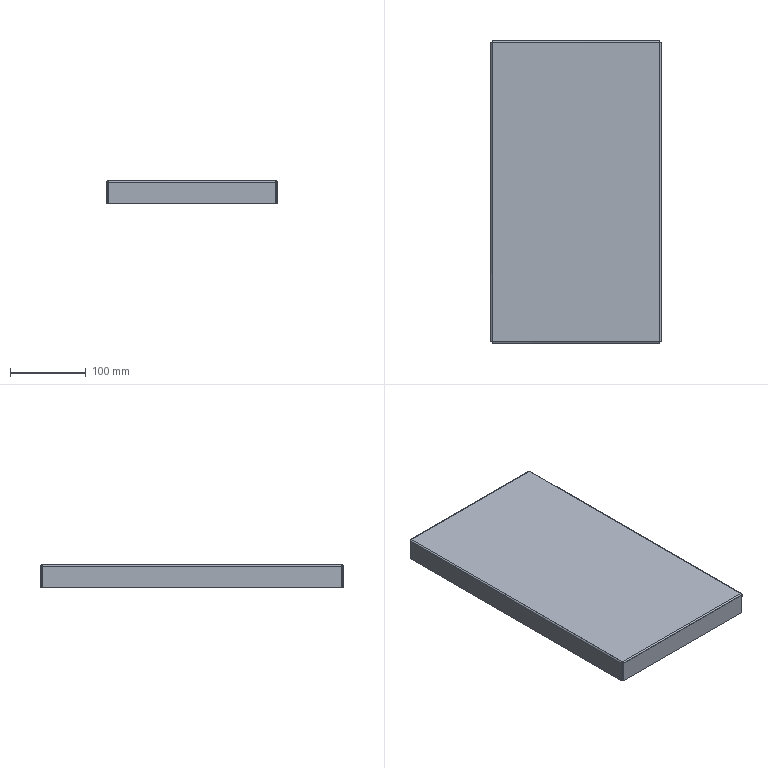Part | 1 solid | 38 faces | box 225 x 400 x 30 mm | volume 149808 mm3 | plane 22 | spline 8 | cylinder 8 | commonest cylinder face diameters 1.465 x4 3.865 x4
STEP:
#1=CARTESIAN_POINT('',(-110.567,-198.067,-1.2));
#2=VERTEX_POINT('',#1);
#3=CARTESIAN_POINT('',(110.567,-198.067,-1.2));
#4=VERTEX_POINT('',#3);
#5=CARTESIAN_POINT('',(-110.593,-198.067,-1.2));
#6=DIRECTION('',(1.,0.,0.));
#7=VECTOR('',#6,1000.);
#8=LINE('',#5,#7);
#9=EDGE_CURVE('',#2,#4,#8,.T.);
#10=ORIENTED_EDGE('',*,*,#9,.F.);
#11=CARTESIAN_POINT('',(-110.567,198.067,-1.2));
#12=VERTEX_POINT('',#11);
#13=CARTESIAN_POINT('',(-110.567,198.093,-1.2));
#14=DIRECTION('',(0.,-1.,0.));
#15=VECTOR('',#14,1000.);
#16=LINE('',#13,#15);
#17=EDGE_CURVE('',#12,#2,#16,.T.);
#18=ORIENTED_EDGE('',*,*,#17,.F.);
#19=CARTESIAN_POINT('',(110.567,198.067,-1.2));
#20=VERTEX_POINT('',#19);
#21=CARTESIAN_POINT('',(110.593,198.067,-1.2));
#22=DIRECTION('',(-1.,0.,0.));
#23=VECTOR('',#22,1000.);
#24=LINE('',#21,#23);
#25=EDGE_CURVE('',#20,#12,#24,.T.);
#26=ORIENTED_EDGE('',*,*,#25,.F.);
#27=CARTESIAN_POINT('',(110.567,-198.093,-1.2));
#28=DIRECTION('',(0.,1.,0.));
#29=VECTOR('',#28,1000.);
#30=LINE('',#27,#29);
#31=EDGE_CURVE('',#4,#20,#30,.T.);
#32=ORIENTED_EDGE('',*,*,#31,.F.);
#33=EDGE_LOOP('',(#10,#18,#26,#32));
#34=FACE_OUTER_BOUND('',#33,.T.);
#35=CARTESIAN_POINT('',(0.,0.,-1.2));
#36=DIRECTION('',(0.,0.,1.));
#37=DIRECTION('',(1.,0.,0.));
#38=AXIS2_PLACEMENT_3D('',#35,#36,#37);
#39=PLANE('',#38);
#40=ADVANCED_FACE('',(#34),#39,.F.);
#41=CARTESIAN_POINT('',(-110.567,198.067,0.));
#42=VERTEX_POINT('',#41);
#43=CARTESIAN_POINT('',(-110.567,-198.067,0.));
#44=VERTEX_POINT('',#43);
#45=CARTESIAN_POINT('',(-110.567,198.093,0.));
#46=DIRECTION('',(0.,-1.,0.));
#47=VECTOR('',#46,1000.);
#48=LINE('',#45,#47);
#49=EDGE_CURVE('',#42,#44,#48,.T.);
#50=ORIENTED_EDGE('',*,*,#49,.T.);
#51=CARTESIAN_POINT('',(110.567,-198.067,0.));
#52=VERTEX_POINT('',#51);
#53=CARTESIAN_POINT('',(-110.593,-198.067,0.));
#54=DIRECTION('',(1.,0.,0.));
#55=VECTOR('',#54,1000.);
#56=LINE('',#53,#55);
#57=EDGE_CURVE('',#44,#52,#56,.T.);
#58=ORIENTED_EDGE('',*,*,#57,.T.);
#59=CARTESIAN_POINT('',(110.567,198.067,0.));
#60=VERTEX_POINT('',#59);
#61=CARTESIAN_POINT('',(110.567,-198.093,0.));
#62=DIRECTION('',(0.,1.,0.));
#63=VECTOR('',#62,1000.);
#64=LINE('',#61,#63);
#65=EDGE_CURVE('',#52,#60,#64,.T.);
#66=ORIENTED_EDGE('',*,*,#65,.T.);
#67=CARTESIAN_POINT('',(110.593,198.067,0.));
#68=DIRECTION('',(-1.,0.,0.));
#69=VECTOR('',#68,1000.);
#70=LINE('',#67,#69);
#71=EDGE_CURVE('',#60,#42,#70,.T.);
#72=ORIENTED_EDGE('',*,*,#71,.T.);
#73=EDGE_LOOP('',(#50,#58,#66,#72));
#74=FACE_OUTER_BOUND('',#73,.T.);
#75=CARTESIAN_POINT('',(0.,0.,0.));
#76=DIRECTION('',(0.,0.,1.));
#77=DIRECTION('',(1.,0.,0.));
#78=AXIS2_PLACEMENT_3D('',#75,#76,#77);
#79=PLANE('',#78);
#80=ADVANCED_FACE('',(#74),#79,.T.);
#81=CARTESIAN_POINT('',(112.5,198.093,-1.933));
#82=VERTEX_POINT('',#81);
#83=CARTESIAN_POINT('',(111.3,198.093,-1.933));
#84=VERTEX_POINT('',#83);
#85=CARTESIAN_POINT('',(111.3,198.093,-1.933));
#86=DIRECTION('',(-1.,0.,0.));
#87=VECTOR('',#86,1000.);
#88=LINE('',#85,#87);
#89=EDGE_CURVE('',#82,#84,#88,.T.);
#90=ORIENTED_EDGE('',*,*,#89,.T.);
#91=CARTESIAN_POINT('',(110.567,198.067,-1.2));
#92=CARTESIAN_POINT('',(110.759,198.072,-1.2));
#93=CARTESIAN_POINT('',(110.95,198.076,-1.279));
#94=CARTESIAN_POINT('',(111.221,198.084,-1.55));
#95=CARTESIAN_POINT('',(111.3,198.089,-1.741));
#96=CARTESIAN_POINT('',(111.3,198.093,-1.933));
#97=B_SPLINE_CURVE_WITH_KNOTS('',3,(#91,#92,#93,#94,#95,#96),.UNSPECIFIED.,.F.,.F.,(4,2,4),(0.,0.5,1.),.UNSPECIFIED.);
#98=EDGE_CURVE('',#20,#84,#97,.T.);
#99=ORIENTED_EDGE('',*,*,#98,.F.);
#100=CARTESIAN_POINT('',(110.567,198.067,-1.2));
#101=DIRECTION('',(0.,0.,1.));
#102=VECTOR('',#101,1000.);
#103=LINE('',#100,#102);
#104=EDGE_CURVE('',#20,#60,#103,.T.);
#105=ORIENTED_EDGE('',*,*,#104,.T.);
#106=CARTESIAN_POINT('',(110.567,198.067,0.));
#107=CARTESIAN_POINT('',(110.82,198.07,0.));
#108=CARTESIAN_POINT('',(111.073,198.072,-0.0503));
#109=CARTESIAN_POINT('',(111.541,198.076,-0.2439));
#110=CARTESIAN_POINT('',(111.755,198.078,-0.3872));
#111=CARTESIAN_POINT('',(112.113,198.082,-0.7449));
#112=CARTESIAN_POINT('',(112.256,198.084,-0.9593));
#113=CARTESIAN_POINT('',(112.45,198.089,-1.427));
#114=CARTESIAN_POINT('',(112.5,198.091,-1.68));
#115=CARTESIAN_POINT('',(112.5,198.093,-1.933));
#116=B_SPLINE_CURVE_WITH_KNOTS('',3,(#106,#107,#108,#109,#110,#111,#112,#113,#114,#115),.UNSPECIFIED.,.F.,.F.,(4,2,2,2,4),(0.,0.25,0.5,0.75,1.),.UNSPECIFIED.);
#117=EDGE_CURVE('',#60,#82,#116,.T.);
#118=ORIENTED_EDGE('',*,*,#117,.T.);
#119=EDGE_LOOP('',(#90,#99,#105,#118));
#120=FACE_OUTER_BOUND('',#119,.T.);
#121=CARTESIAN_POINT('',(110.567,198.067,0.012));
#122=CARTESIAN_POINT('',(110.822,198.07,0.012));
#123=CARTESIAN_POINT('',(111.076,198.072,-0.03861));
#124=CARTESIAN_POINT('',(111.547,198.076,-0.2334));
#125=CARTESIAN_POINT('',(111.762,198.078,-0.3776));
#126=CARTESIAN_POINT('',(112.122,198.082,-0.7376));
#127=CARTESIAN_POINT('',(112.267,198.084,-0.9533));
#128=CARTESIAN_POINT('',(112.461,198.089,-1.424));
#129=CARTESIAN_POINT('',(112.512,198.091,-1.678));
#130=CARTESIAN_POINT('',(112.512,198.093,-1.933));
#131=CARTESIAN_POINT('',(110.567,198.067,0.));
#132=CARTESIAN_POINT('',(110.82,198.07,0.));
#133=CARTESIAN_POINT('',(111.073,198.072,-0.0503));
#134=CARTESIAN_POINT('',(111.541,198.076,-0.2439));
#135=CARTESIAN_POINT('',(111.755,198.078,-0.3872));
#136=CARTESIAN_POINT('',(112.113,198.082,-0.7449));
#137=CARTESIAN_POINT('',(112.256,198.084,-0.9593));
#138=CARTESIAN_POINT('',(112.45,198.089,-1.427));
#139=CARTESIAN_POINT('',(112.5,198.091,-1.68));
#140=CARTESIAN_POINT('',(112.5,198.093,-1.933));
#141=CARTESIAN_POINT('',(110.567,198.067,-1.2));
#142=CARTESIAN_POINT('',(110.663,198.07,-1.2));
#143=CARTESIAN_POINT('',(110.759,198.072,-1.219));
#144=CARTESIAN_POINT('',(110.936,198.076,-1.292));
#145=CARTESIAN_POINT('',(111.018,198.078,-1.347));
#146=CARTESIAN_POINT('',(111.153,198.082,-1.482));
#147=CARTESIAN_POINT('',(111.208,198.084,-1.564));
#148=CARTESIAN_POINT('',(111.281,198.089,-1.741));
#149=CARTESIAN_POINT('',(111.3,198.091,-1.837));
#150=CARTESIAN_POINT('',(111.3,198.093,-1.933));
#151=CARTESIAN_POINT('',(110.567,198.067,-1.212));
#152=CARTESIAN_POINT('',(110.662,198.07,-1.212));
#153=CARTESIAN_POINT('',(110.756,198.072,-1.231));
#154=CARTESIAN_POINT('',(110.93,198.076,-1.303));
#155=CARTESIAN_POINT('',(111.01,198.078,-1.356));
#156=CARTESIAN_POINT('',(111.144,198.082,-1.49));
#157=CARTESIAN_POINT('',(111.197,198.084,-1.57));
#158=CARTESIAN_POINT('',(111.269,198.089,-1.744));
#159=CARTESIAN_POINT('',(111.288,198.091,-1.838));
#160=CARTESIAN_POINT('',(111.288,198.093,-1.933));
#161=B_SPLINE_SURFACE_WITH_KNOTS('',1,3,((#121,#122,#123,#124,#125,#126,#127,#128,#129,#130),(#131,#132,#133,#134,#135,#136,#137,#138,#139,#140),(#141,#142,#143,#144,#145,#146,#147,#148,#149,#150),(#151,#152,#153,#154,#155,#156,#157,#158,#159,#160)),.UNSPECIFIED.,.F.,.F.,.F.,(2,1,1,2),(4,2,2,2,4),(-0.01,0.,1.,1.01),(0.,0.25,0.5,0.75,1.),.UNSPECIFIED.);
#162=ADVANCED_FACE('',(#120),#161,.F.);
#163=CARTESIAN_POINT('',(111.3,-198.093,-1.933));
#164=VERTEX_POINT('',#163);
#165=CARTESIAN_POINT('',(111.3,-198.093,-1.933));
#166=CARTESIAN_POINT('',(111.3,-198.089,-1.741));
#167=CARTESIAN_POINT('',(111.221,-198.084,-1.55));
#168=CARTESIAN_POINT('',(110.95,-198.076,-1.279));
#169=CARTESIAN_POINT('',(110.759,-198.072,-1.2));
#170=CARTESIAN_POINT('',(110.567,-198.067,-1.2));
#171=B_SPLINE_CURVE_WITH_KNOTS('',3,(#165,#166,#167,#168,#169,#170),.UNSPECIFIED.,.F.,.F.,(4,2,4),(0.,0.5,1.),.UNSPECIFIED.);
#172=EDGE_CURVE('',#164,#4,#171,.T.);
#173=ORIENTED_EDGE('',*,*,#172,.F.);
#174=CARTESIAN_POINT('',(112.5,-198.093,-1.933));
#175=VERTEX_POINT('',#174);
#176=CARTESIAN_POINT('',(111.3,-198.093,-1.933));
#177=DIRECTION('',(-1.,0.,0.));
#178=VECTOR('',#177,1000.);
#179=LINE('',#176,#178);
#180=EDGE_CURVE('',#175,#164,#179,.T.);
#181=ORIENTED_EDGE('',*,*,#180,.F.);
#182=CARTESIAN_POINT('',(112.5,-198.093,-1.933));
#183=CARTESIAN_POINT('',(112.5,-198.091,-1.68));
#184=CARTESIAN_POINT('',(112.45,-198.089,-1.427));
#185=CARTESIAN_POINT('',(112.256,-198.084,-0.9593));
#186=CARTESIAN_POINT('',(112.113,-198.082,-0.7449));
#187=CARTESIAN_POINT('',(111.755,-198.078,-0.3872));
#188=CARTESIAN_POINT('',(111.541,-198.076,-0.2439));
#189=CARTESIAN_POINT('',(111.073,-198.072,-0.0503));
#190=CARTESIAN_POINT('',(110.82,-198.07,0.));
#191=CARTESIAN_POINT('',(110.567,-198.067,0.));
#192=B_SPLINE_CURVE_WITH_KNOTS('',3,(#182,#183,#184,#185,#186,#187,#188,#189,#190,#191),.UNSPECIFIED.,.F.,.F.,(4,2,2,2,4),(0.,0.25,0.5,0.75,1.),.UNSPECIFIED.);
#193=EDGE_CURVE('',#175,#52,#192,.T.);
#194=ORIENTED_EDGE('',*,*,#193,.T.);
#195=CARTESIAN_POINT('',(110.567,-198.067,-1.2));
#196=DIRECTION('',(0.,0.,1.));
#197=VECTOR('',#196,1000.);
#198=LINE('',#195,#197);
#199=EDGE_CURVE('',#4,#52,#198,.T.);
#200=ORIENTED_EDGE('',*,*,#199,.F.);
#201=EDGE_LOOP('',(#173,#181,#194,#200));
#202=FACE_OUTER_BOUND('',#201,.T.);
#203=CARTESIAN_POINT('',(112.512,-198.093,-1.933));
#204=CARTESIAN_POINT('',(112.512,-198.091,-1.678));
#205=CARTESIAN_POINT('',(112.461,-198.089,-1.424));
#206=CARTESIAN_POINT('',(112.267,-198.084,-0.9533));
#207=CARTESIAN_POINT('',(112.122,-198.082,-0.7376));
#208=CARTESIAN_POINT('',(111.762,-198.078,-0.3776));
#209=CARTESIAN_POINT('',(111.547,-198.076,-0.2334));
#210=CARTESIAN_POINT('',(111.076,-198.072,-0.03861));
#211=CARTESIAN_POINT('',(110.822,-198.07,0.012));
#212=CARTESIAN_POINT('',(110.567,-198.067,0.012));
#213=CARTESIAN_POINT('',(112.5,-198.093,-1.933));
#214=CARTESIAN_POINT('',(112.5,-198.091,-1.68));
#215=CARTESIAN_POINT('',(112.45,-198.089,-1.427));
#216=CARTESIAN_POINT('',(112.256,-198.084,-0.9593));
#217=CARTESIAN_POINT('',(112.113,-198.082,-0.7449));
#218=CARTESIAN_POINT('',(111.755,-198.078,-0.3872));
#219=CARTESIAN_POINT('',(111.541,-198.076,-0.2439));
#220=CARTESIAN_POINT('',(111.073,-198.072,-0.0503));
#221=CARTESIAN_POINT('',(110.82,-198.07,0.));
#222=CARTESIAN_POINT('',(110.567,-198.067,0.));
#223=CARTESIAN_POINT('',(111.3,-198.093,-1.933));
#224=CARTESIAN_POINT('',(111.3,-198.091,-1.837));
#225=CARTESIAN_POINT('',(111.281,-198.089,-1.741));
#226=CARTESIAN_POINT('',(111.208,-198.084,-1.564));
#227=CARTESIAN_POINT('',(111.153,-198.082,-1.482));
#228=CARTESIAN_POINT('',(111.018,-198.078,-1.347));
#229=CARTESIAN_POINT('',(110.936,-198.076,-1.292));
#230=CARTESIAN_POINT('',(110.759,-198.072,-1.219));
#231=CARTESIAN_POINT('',(110.663,-198.07,-1.2));
#232=CARTESIAN_POINT('',(110.567,-198.067,-1.2));
#233=CARTESIAN_POINT('',(111.288,-198.093,-1.933));
#234=CARTESIAN_POINT('',(111.288,-198.091,-1.838));
#235=CARTESIAN_POINT('',(111.269,-198.089,-1.744));
#236=CARTESIAN_POINT('',(111.197,-198.084,-1.57));
#237=CARTESIAN_POINT('',(111.144,-198.082,-1.49));
#238=CARTESIAN_POINT('',(111.01,-198.078,-1.356));
#239=CARTESIAN_POINT('',(110.93,-198.076,-1.303));
#240=CARTESIAN_POINT('',(110.756,-198.072,-1.231));
#241=CARTESIAN_POINT('',(110.662,-198.07,-1.212));
#242=CARTESIAN_POINT('',(110.567,-198.067,-1.212));
#243=B_SPLINE_SURFACE_WITH_KNOTS('',1,3,((#203,#204,#205,#206,#207,#208,#209,#210,#211,#212),(#213,#214,#215,#216,#217,#218,#219,#220,#221,#222),(#223,#224,#225,#226,#227,#228,#229,#230,#231,#232),(#233,#234,#235,#236,#237,#238,#239,#240,#241,#242)),.UNSPECIFIED.,.F.,.F.,.F.,(2,1,1,2),(4,2,2,2,4),(-0.01,0.,1.,1.01),(0.,0.25,0.5,0.75,1.),.UNSPECIFIED.);
#244=ADVANCED_FACE('',(#202),#243,.F.);
#245=ORIENTED_EDGE('',*,*,#65,.F.);
#246=ORIENTED_EDGE('',*,*,#193,.F.);
#247=CARTESIAN_POINT('',(112.5,0.,-1.933));
#248=DIRECTION('',(0.,-1.,0.));
#249=VECTOR('',#248,1000.);
#250=LINE('',#247,#249);
#251=EDGE_CURVE('',#82,#175,#250,.T.);
#252=ORIENTED_EDGE('',*,*,#251,.F.);
#253=ORIENTED_EDGE('',*,*,#117,.F.);
#254=EDGE_LOOP('',(#245,#246,#252,#253));
#255=FACE_OUTER_BOUND('',#254,.T.);
#256=CARTESIAN_POINT('',(110.567,-198.093,-1.933));
#257=DIRECTION('',(0.,-1.,0.));
#258=DIRECTION('',(1.,0.,0.));
#259=AXIS2_PLACEMENT_3D('',#256,#257,#258);
#260=CYLINDRICAL_SURFACE('',#259,1.933);
#261=ADVANCED_FACE('',(#255),#260,.T.);
#262=ORIENTED_EDGE('',*,*,#31,.T.);
#263=ORIENTED_EDGE('',*,*,#98,.T.);
#264=CARTESIAN_POINT('',(111.3,200.,-1.933));
#265=DIRECTION('',(0.,-1.,0.));
#266=VECTOR('',#265,1000.);
#267=LINE('',#264,#266);
#268=EDGE_CURVE('',#84,#164,#267,.T.);
#269=ORIENTED_EDGE('',*,*,#268,.T.);
#270=ORIENTED_EDGE('',*,*,#172,.T.);
#271=EDGE_LOOP('',(#262,#263,#269,#270));
#272=FACE_OUTER_BOUND('',#271,.T.);
#273=CARTESIAN_POINT('',(110.567,-198.093,-1.933));
#274=DIRECTION('',(0.,-1.,0.));
#275=DIRECTION('',(1.,0.,0.));
#276=AXIS2_PLACEMENT_3D('',#273,#274,#275);
#277=CYLINDRICAL_SURFACE('',#276,0.7326);
#278=ADVANCED_FACE('',(#272),#277,.F.);
#279=CARTESIAN_POINT('',(111.3,198.093,-30.));
#280=VERTEX_POINT('',#279);
#281=CARTESIAN_POINT('',(112.5,198.093,-30.));
#282=VERTEX_POINT('',#281);
#283=CARTESIAN_POINT('',(112.5,198.093,-30.));
#284=DIRECTION('',(1.,0.,0.));
#285=VECTOR('',#284,1000.);
#286=LINE('',#283,#285);
#287=EDGE_CURVE('',#280,#282,#286,.T.);
#288=ORIENTED_EDGE('',*,*,#287,.F.);
#289=CARTESIAN_POINT('',(111.3,198.093,0.));
#290=DIRECTION('',(0.,0.,-1.));
#291=VECTOR('',#290,1000.);
#292=LINE('',#289,#291);
#293=EDGE_CURVE('',#84,#280,#292,.T.);
#294=ORIENTED_EDGE('',*,*,#293,.F.);
#295=ORIENTED_EDGE('',*,*,#89,.F.);
#296=CARTESIAN_POINT('',(112.5,198.093,0.));
#297=DIRECTION('',(0.,0.,1.));
#298=VECTOR('',#297,1000.);
#299=LINE('',#296,#298);
#300=EDGE_CURVE('',#282,#82,#299,.T.);
#301=ORIENTED_EDGE('',*,*,#300,.F.);
#302=EDGE_LOOP('',(#288,#294,#295,#301));
#303=FACE_OUTER_BOUND('',#302,.T.);
#304=CARTESIAN_POINT('',(111.3,198.093,-1.2));
#305=DIRECTION('',(0.,1.,0.));
#306=DIRECTION('',(0.,0.,-1.));
#307=AXIS2_PLACEMENT_3D('',#304,#305,#306);
#308=PLANE('',#307);
#309=ADVANCED_FACE('',(#303),#308,.T.);
#310=CARTESIAN_POINT('',(112.5,-198.093,-30.));
#311=VERTEX_POINT('',#310);
#312=CARTESIAN_POINT('',(112.5,-198.093,-1.2));
#313=DIRECTION('',(0.,0.,1.));
#314=VECTOR('',#313,1000.);
#315=LINE('',#312,#314);
#316=EDGE_CURVE('',#311,#175,#315,.T.);
#317=ORIENTED_EDGE('',*,*,#316,.F.);
#318=CARTESIAN_POINT('',(112.5,-200.,-30.));
#319=DIRECTION('',(0.,-1.,0.));
#320=VECTOR('',#319,1000.);
#321=LINE('',#318,#320);
#322=EDGE_CURVE('',#282,#311,#321,.T.);
#323=ORIENTED_EDGE('',*,*,#322,.F.);
#324=ORIENTED_EDGE('',*,*,#300,.T.);
#325=ORIENTED_EDGE('',*,*,#251,.T.);
#326=EDGE_LOOP('',(#317,#323,#324,#325));
#327=FACE_OUTER_BOUND('',#326,.T.);
#328=CARTESIAN_POINT('',(112.5,0.,0.));
#329=DIRECTION('',(1.,0.,0.));
#330=DIRECTION('',(0.,0.,1.));
#331=AXIS2_PLACEMENT_3D('',#328,#329,#330);
#332=PLANE('',#331);
#333=ADVANCED_FACE('',(#327),#332,.T.);
#334=CARTESIAN_POINT('',(111.3,-198.093,-30.));
#335=VERTEX_POINT('',#334);
#336=CARTESIAN_POINT('',(111.3,0.,-30.));
#337=DIRECTION('',(0.,-1.,0.));
#338=VECTOR('',#337,1000.);
#339=LINE('',#336,#338);
#340=EDGE_CURVE('',#280,#335,#339,.T.);
#341=ORIENTED_EDGE('',*,*,#340,.T.);
#342=CARTESIAN_POINT('',(111.3,-198.093,-1.2));
#343=DIRECTION('',(0.,0.,-1.));
#344=VECTOR('',#343,1000.);
#345=LINE('',#342,#344);
#346=EDGE_CURVE('',#164,#335,#345,.T.);
#347=ORIENTED_EDGE('',*,*,#346,.F.);
#348=ORIENTED_EDGE('',*,*,#268,.F.);
#349=ORIENTED_EDGE('',*,*,#293,.T.);
#350=EDGE_LOOP('',(#341,#347,#348,#349));
#351=FACE_OUTER_BOUND('',#350,.T.);
#352=CARTESIAN_POINT('',(111.3,0.,0.));
#353=DIRECTION('',(1.,0.,0.));
#354=DIRECTION('',(0.,0.,1.));
#355=AXIS2_PLACEMENT_3D('',#352,#353,#354);
#356=PLANE('',#355);
#357=ADVANCED_FACE('',(#351),#356,.F.);
#358=CARTESIAN_POINT('',(111.3,-198.093,-30.));
#359=DIRECTION('',(1.,0.,0.));
#360=VECTOR('',#359,1000.);
#361=LINE('',#358,#360);
#362=EDGE_CURVE('',#335,#311,#361,.T.);
#363=ORIENTED_EDGE('',*,*,#362,.F.);
#364=ORIENTED_EDGE('',*,*,#340,.F.);
#365=ORIENTED_EDGE('',*,*,#287,.T.);
#366=ORIENTED_EDGE('',*,*,#322,.T.);
#367=EDGE_LOOP('',(#363,#364,#365,#366));
#368=FACE_OUTER_BOUND('',#367,.T.);
#369=CARTESIAN_POINT('',(112.5,-200.,-30.));
#370=DIRECTION('',(0.,0.,-1.));
#371=DIRECTION('',(0.,-1.,0.));
#372=AXIS2_PLACEMENT_3D('',#369,#370,#371);
#373=PLANE('',#372);
#374=ADVANCED_FACE('',(#368),#373,.T.);
#375=ORIENTED_EDGE('',*,*,#346,.T.);
#376=ORIENTED_EDGE('',*,*,#362,.T.);
#377=ORIENTED_EDGE('',*,*,#316,.T.);
#378=ORIENTED_EDGE('',*,*,#180,.T.);
#379=EDGE_LOOP('',(#375,#376,#377,#378));
#380=FACE_OUTER_BOUND('',#379,.T.);
#381=CARTESIAN_POINT('',(111.3,-198.093,-1.2));
#382=DIRECTION('',(0.,1.,0.));
#383=DIRECTION('',(0.,0.,-1.));
#384=AXIS2_PLACEMENT_3D('',#381,#382,#383);
#385=PLANE('',#384);
#386=ADVANCED_FACE('',(#380),#385,.F.);
#387=CARTESIAN_POINT('',(-110.593,200.,-1.933));
#388=VERTEX_POINT('',#387);
#389=CARTESIAN_POINT('',(-110.593,198.8,-1.933));
#390=VERTEX_POINT('',#389);
#391=CARTESIAN_POINT('',(-110.593,198.8,-1.933));
#392=DIRECTION('',(0.,-1.,0.));
#393=VECTOR('',#392,1000.);
#394=LINE('',#391,#393);
#395=EDGE_CURVE('',#388,#390,#394,.T.);
#396=ORIENTED_EDGE('',*,*,#395,.T.);
#397=CARTESIAN_POINT('',(-110.567,198.067,-1.2));
#398=CARTESIAN_POINT('',(-110.572,198.259,-1.2));
#399=CARTESIAN_POINT('',(-110.576,198.45,-1.279));
#400=CARTESIAN_POINT('',(-110.584,198.721,-1.55));
#401=CARTESIAN_POINT('',(-110.589,198.8,-1.741));
#402=CARTESIAN_POINT('',(-110.593,198.8,-1.933));
#403=B_SPLINE_CURVE_WITH_KNOTS('',3,(#397,#398,#399,#400,#401,#402),.UNSPECIFIED.,.F.,.F.,(4,2,4),(0.,0.5,1.),.UNSPECIFIED.);
#404=EDGE_CURVE('',#12,#390,#403,.T.);
#405=ORIENTED_EDGE('',*,*,#404,.F.);
#406=CARTESIAN_POINT('',(-110.567,198.067,-1.2));
#407=DIRECTION('',(0.,0.,1.));
#408=VECTOR('',#407,1000.);
#409=LINE('',#406,#408);
#410=EDGE_CURVE('',#12,#42,#409,.T.);
#411=ORIENTED_EDGE('',*,*,#410,.T.);
#412=CARTESIAN_POINT('',(-110.567,198.067,0.));
#413=CARTESIAN_POINT('',(-110.57,198.32,0.));
#414=CARTESIAN_POINT('',(-110.572,198.573,-0.0503));
#415=CARTESIAN_POINT('',(-110.576,199.041,-0.2439));
#416=CARTESIAN_POINT('',(-110.578,199.255,-0.3872));
#417=CARTESIAN_POINT('',(-110.582,199.613,-0.7449));
#418=CARTESIAN_POINT('',(-110.584,199.756,-0.9593));
#419=CARTESIAN_POINT('',(-110.589,199.95,-1.427));
#420=CARTESIAN_POINT('',(-110.591,200.,-1.68));
#421=CARTESIAN_POINT('',(-110.593,200.,-1.933));
#422=B_SPLINE_CURVE_WITH_KNOTS('',3,(#412,#413,#414,#415,#416,#417,#418,#419,#420,#421),.UNSPECIFIED.,.F.,.F.,(4,2,2,2,4),(0.,0.25,0.5,0.75,1.),.UNSPECIFIED.);
#423=EDGE_CURVE('',#42,#388,#422,.T.);
#424=ORIENTED_EDGE('',*,*,#423,.T.);
#425=EDGE_LOOP('',(#396,#405,#411,#424));
#426=FACE_OUTER_BOUND('',#425,.T.);
#427=CARTESIAN_POINT('',(-110.567,198.067,0.012));
#428=CARTESIAN_POINT('',(-110.57,198.322,0.012));
#429=CARTESIAN_POINT('',(-110.572,198.576,-0.03861));
#430=CARTESIAN_POINT('',(-110.576,199.047,-0.2334));
#431=CARTESIAN_POINT('',(-110.578,199.262,-0.3776));
#432=CARTESIAN_POINT('',(-110.582,199.622,-0.7376));
#433=CARTESIAN_POINT('',(-110.584,199.767,-0.9533));
#434=CARTESIAN_POINT('',(-110.589,199.961,-1.424));
#435=CARTESIAN_POINT('',(-110.591,200.012,-1.678));
#436=CARTESIAN_POINT('',(-110.593,200.012,-1.933));
#437=CARTESIAN_POINT('',(-110.567,198.067,0.));
#438=CARTESIAN_POINT('',(-110.57,198.32,0.));
#439=CARTESIAN_POINT('',(-110.572,198.573,-0.0503));
#440=CARTESIAN_POINT('',(-110.576,199.041,-0.2439));
#441=CARTESIAN_POINT('',(-110.578,199.255,-0.3872));
#442=CARTESIAN_POINT('',(-110.582,199.613,-0.7449));
#443=CARTESIAN_POINT('',(-110.584,199.756,-0.9593));
#444=CARTESIAN_POINT('',(-110.589,199.95,-1.427));
#445=CARTESIAN_POINT('',(-110.591,200.,-1.68));
#446=CARTESIAN_POINT('',(-110.593,200.,-1.933));
#447=CARTESIAN_POINT('',(-110.567,198.067,-1.2));
#448=CARTESIAN_POINT('',(-110.57,198.163,-1.2));
#449=CARTESIAN_POINT('',(-110.572,198.259,-1.219));
#450=CARTESIAN_POINT('',(-110.576,198.436,-1.292));
#451=CARTESIAN_POINT('',(-110.578,198.518,-1.347));
#452=CARTESIAN_POINT('',(-110.582,198.653,-1.482));
#453=CARTESIAN_POINT('',(-110.584,198.708,-1.564));
#454=CARTESIAN_POINT('',(-110.589,198.781,-1.741));
#455=CARTESIAN_POINT('',(-110.591,198.8,-1.837));
#456=CARTESIAN_POINT('',(-110.593,198.8,-1.933));
#457=CARTESIAN_POINT('',(-110.567,198.067,-1.212));
#458=CARTESIAN_POINT('',(-110.57,198.162,-1.212));
#459=CARTESIAN_POINT('',(-110.572,198.256,-1.231));
#460=CARTESIAN_POINT('',(-110.576,198.43,-1.303));
#461=CARTESIAN_POINT('',(-110.578,198.51,-1.356));
#462=CARTESIAN_POINT('',(-110.582,198.644,-1.49));
#463=CARTESIAN_POINT('',(-110.584,198.697,-1.57));
#464=CARTESIAN_POINT('',(-110.589,198.769,-1.744));
#465=CARTESIAN_POINT('',(-110.591,198.788,-1.838));
#466=CARTESIAN_POINT('',(-110.593,198.788,-1.933));
#467=B_SPLINE_SURFACE_WITH_KNOTS('',1,3,((#427,#428,#429,#430,#431,#432,#433,#434,#435,#436),(#437,#438,#439,#440,#441,#442,#443,#444,#445,#446),(#447,#448,#449,#450,#451,#452,#453,#454,#455,#456),(#457,#458,#459,#460,#461,#462,#463,#464,#465,#466)),.UNSPECIFIED.,.F.,.F.,.F.,(2,1,1,2),(4,2,2,2,4),(-0.01,0.,1.,1.01),(0.,0.25,0.5,0.75,1.),.UNSPECIFIED.);
#468=ADVANCED_FACE('',(#426),#467,.F.);
#469=CARTESIAN_POINT('',(110.593,198.8,-1.933));
#470=VERTEX_POINT('',#469);
#471=CARTESIAN_POINT('',(110.593,198.8,-1.933));
#472=CARTESIAN_POINT('',(110.589,198.8,-1.741));
#473=CARTESIAN_POINT('',(110.584,198.721,-1.55));
#474=CARTESIAN_POINT('',(110.576,198.45,-1.279));
#475=CARTESIAN_POINT('',(110.572,198.259,-1.2));
#476=CARTESIAN_POINT('',(110.567,198.067,-1.2));
#477=B_SPLINE_CURVE_WITH_KNOTS('',3,(#471,#472,#473,#474,#475,#476),.UNSPECIFIED.,.F.,.F.,(4,2,4),(0.,0.5,1.),.UNSPECIFIED.);
#478=EDGE_CURVE('',#470,#20,#477,.T.);
#479=ORIENTED_EDGE('',*,*,#478,.F.);
#480=CARTESIAN_POINT('',(110.593,200.,-1.933));
#481=VERTEX_POINT('',#480);
#482=CARTESIAN_POINT('',(110.593,198.8,-1.933));
#483=DIRECTION('',(0.,-1.,0.));
#484=VECTOR('',#483,1000.);
#485=LINE('',#482,#484);
#486=EDGE_CURVE('',#481,#470,#485,.T.);
#487=ORIENTED_EDGE('',*,*,#486,.F.);
#488=CARTESIAN_POINT('',(110.593,200.,-1.933));
#489=CARTESIAN_POINT('',(110.591,200.,-1.68));
#490=CARTESIAN_POINT('',(110.589,199.95,-1.427));
#491=CARTESIAN_POINT('',(110.584,199.756,-0.9593));
#492=CARTESIAN_POINT('',(110.582,199.613,-0.7449));
#493=CARTESIAN_POINT('',(110.578,199.255,-0.3872));
#494=CARTESIAN_POINT('',(110.576,199.041,-0.2439));
#495=CARTESIAN_POINT('',(110.572,198.573,-0.0503));
#496=CARTESIAN_POINT('',(110.57,198.32,0.));
#497=CARTESIAN_POINT('',(110.567,198.067,0.));
#498=B_SPLINE_CURVE_WITH_KNOTS('',3,(#488,#489,#490,#491,#492,#493,#494,#495,#496,#497),.UNSPECIFIED.,.F.,.F.,(4,2,2,2,4),(0.,0.25,0.5,0.75,1.),.UNSPECIFIED.);
#499=EDGE_CURVE('',#481,#60,#498,.T.);
#500=ORIENTED_EDGE('',*,*,#499,.T.);
#501=ORIENTED_EDGE('',*,*,#104,.F.);
#502=EDGE_LOOP('',(#479,#487,#500,#501));
#503=FACE_OUTER_BOUND('',#502,.T.);
#504=CARTESIAN_POINT('',(110.593,200.012,-1.933));
#505=CARTESIAN_POINT('',(110.591,200.012,-1.678));
#506=CARTESIAN_POINT('',(110.589,199.961,-1.424));
#507=CARTESIAN_POINT('',(110.584,199.767,-0.9533));
#508=CARTESIAN_POINT('',(110.582,199.622,-0.7376));
#509=CARTESIAN_POINT('',(110.578,199.262,-0.3776));
#510=CARTESIAN_POINT('',(110.576,199.047,-0.2334));
#511=CARTESIAN_POINT('',(110.572,198.576,-0.03861));
#512=CARTESIAN_POINT('',(110.57,198.322,0.012));
#513=CARTESIAN_POINT('',(110.567,198.067,0.012));
#514=CARTESIAN_POINT('',(110.593,200.,-1.933));
#515=CARTESIAN_POINT('',(110.591,200.,-1.68));
#516=CARTESIAN_POINT('',(110.589,199.95,-1.427));
#517=CARTESIAN_POINT('',(110.584,199.756,-0.9593));
#518=CARTESIAN_POINT('',(110.582,199.613,-0.7449));
#519=CARTESIAN_POINT('',(110.578,199.255,-0.3872));
#520=CARTESIAN_POINT('',(110.576,199.041,-0.2439));
#521=CARTESIAN_POINT('',(110.572,198.573,-0.0503));
#522=CARTESIAN_POINT('',(110.57,198.32,0.));
#523=CARTESIAN_POINT('',(110.567,198.067,0.));
#524=CARTESIAN_POINT('',(110.593,198.8,-1.933));
#525=CARTESIAN_POINT('',(110.591,198.8,-1.837));
#526=CARTESIAN_POINT('',(110.589,198.781,-1.741));
#527=CARTESIAN_POINT('',(110.584,198.708,-1.564));
#528=CARTESIAN_POINT('',(110.582,198.653,-1.482));
#529=CARTESIAN_POINT('',(110.578,198.518,-1.347));
#530=CARTESIAN_POINT('',(110.576,198.436,-1.292));
#531=CARTESIAN_POINT('',(110.572,198.259,-1.219));
#532=CARTESIAN_POINT('',(110.57,198.163,-1.2));
#533=CARTESIAN_POINT('',(110.567,198.067,-1.2));
#534=CARTESIAN_POINT('',(110.593,198.788,-1.933));
#535=CARTESIAN_POINT('',(110.591,198.788,-1.838));
#536=CARTESIAN_POINT('',(110.589,198.769,-1.744));
#537=CARTESIAN_POINT('',(110.584,198.697,-1.57));
#538=CARTESIAN_POINT('',(110.582,198.644,-1.49));
#539=CARTESIAN_POINT('',(110.578,198.51,-1.356));
#540=CARTESIAN_POINT('',(110.576,198.43,-1.303));
#541=CARTESIAN_POINT('',(110.572,198.256,-1.231));
#542=CARTESIAN_POINT('',(110.57,198.162,-1.212));
#543=CARTESIAN_POINT('',(110.567,198.067,-1.212));
#544=B_SPLINE_SURFACE_WITH_KNOTS('',1,3,((#504,#505,#506,#507,#508,#509,#510,#511,#512,#513),(#514,#515,#516,#517,#518,#519,#520,#521,#522,#523),(#524,#525,#526,#527,#528,#529,#530,#531,#532,#533),(#534,#535,#536,#537,#538,#539,#540,#541,#542,#543)),.UNSPECIFIED.,.F.,.F.,.F.,(2,1,1,2),(4,2,2,2,4),(-0.01,0.,1.,1.01),(0.,0.25,0.5,0.75,1.),.UNSPECIFIED.);
#545=ADVANCED_FACE('',(#503),#544,.F.);
#546=ORIENTED_EDGE('',*,*,#71,.F.);
#547=ORIENTED_EDGE('',*,*,#499,.F.);
#548=CARTESIAN_POINT('',(-112.5,200.,-1.933));
#549=DIRECTION('',(-1.,0.,0.));
#550=VECTOR('',#549,1000.);
#551=LINE('',#548,#550);
#552=EDGE_CURVE('',#481,#388,#551,.T.);
#553=ORIENTED_EDGE('',*,*,#552,.T.);
#554=ORIENTED_EDGE('',*,*,#423,.F.);
#555=EDGE_LOOP('',(#546,#547,#553,#554));
#556=FACE_OUTER_BOUND('',#555,.T.);
#557=CARTESIAN_POINT('',(110.593,198.067,-1.933));
#558=DIRECTION('',(1.,0.,0.));
#559=DIRECTION('',(0.,1.,0.));
#560=AXIS2_PLACEMENT_3D('',#557,#558,#559);
#561=CYLINDRICAL_SURFACE('',#560,1.933);
#562=ADVANCED_FACE('',(#556),#561,.T.);
#563=ORIENTED_EDGE('',*,*,#25,.T.);
#564=ORIENTED_EDGE('',*,*,#404,.T.);
#565=CARTESIAN_POINT('',(-112.5,198.8,-1.933));
#566=DIRECTION('',(1.,0.,0.));
#567=VECTOR('',#566,1000.);
#568=LINE('',#565,#567);
#569=EDGE_CURVE('',#390,#470,#568,.T.);
#570=ORIENTED_EDGE('',*,*,#569,.T.);
#571=ORIENTED_EDGE('',*,*,#478,.T.);
#572=EDGE_LOOP('',(#563,#564,#570,#571));
#573=FACE_OUTER_BOUND('',#572,.T.);
#574=CARTESIAN_POINT('',(110.593,198.067,-1.933));
#575=DIRECTION('',(1.,0.,0.));
#576=DIRECTION('',(0.,1.,0.));
#577=AXIS2_PLACEMENT_3D('',#574,#575,#576);
#578=CYLINDRICAL_SURFACE('',#577,0.7326);
#579=ADVANCED_FACE('',(#573),#578,.F.);
#580=CARTESIAN_POINT('',(-110.593,198.8,-30.));
#581=VERTEX_POINT('',#580);
#582=CARTESIAN_POINT('',(-110.593,200.,-30.));
#583=VERTEX_POINT('',#582);
#584=CARTESIAN_POINT('',(-110.593,200.,-30.));
#585=DIRECTION('',(0.,1.,0.));
#586=VECTOR('',#585,1000.);
#587=LINE('',#584,#586);
#588=EDGE_CURVE('',#581,#583,#587,.T.);
#589=ORIENTED_EDGE('',*,*,#588,.F.);
#590=CARTESIAN_POINT('',(-110.593,198.8,0.));
#591=DIRECTION('',(0.,0.,-1.));
#592=VECTOR('',#591,1000.);
#593=LINE('',#590,#592);
#594=EDGE_CURVE('',#390,#581,#593,.T.);
#595=ORIENTED_EDGE('',*,*,#594,.F.);
#596=ORIENTED_EDGE('',*,*,#395,.F.);
#597=CARTESIAN_POINT('',(-110.593,200.,-1.2));
#598=DIRECTION('',(0.,0.,-1.));
#599=VECTOR('',#598,1000.);
#600=LINE('',#597,#599);
#601=EDGE_CURVE('',#388,#583,#600,.T.);
#602=ORIENTED_EDGE('',*,*,#601,.T.);
#603=EDGE_LOOP('',(#589,#595,#596,#602));
#604=FACE_OUTER_BOUND('',#603,.T.);
#605=CARTESIAN_POINT('',(-110.593,198.8,-1.2));
#606=DIRECTION('',(-1.,0.,0.));
#607=DIRECTION('',(0.,0.,1.));
#608=AXIS2_PLACEMENT_3D('',#605,#606,#607);
#609=PLANE('',#608);
#610=ADVANCED_FACE('',(#604),#609,.T.);
#611=ORIENTED_EDGE('',*,*,#552,.F.);
#612=CARTESIAN_POINT('',(110.593,200.,-30.));
#613=VERTEX_POINT('',#612);
#614=CARTESIAN_POINT('',(110.593,200.,0.));
#615=DIRECTION('',(0.,0.,-1.));
#616=VECTOR('',#615,1000.);
#617=LINE('',#614,#616);
#618=EDGE_CURVE('',#481,#613,#617,.T.);
#619=ORIENTED_EDGE('',*,*,#618,.T.);
#620=CARTESIAN_POINT('',(-112.5,200.,-30.));
#621=DIRECTION('',(1.,0.,0.));
#622=VECTOR('',#621,1000.);
#623=LINE('',#620,#622);
#624=EDGE_CURVE('',#583,#613,#623,.T.);
#625=ORIENTED_EDGE('',*,*,#624,.F.);
#626=ORIENTED_EDGE('',*,*,#601,.F.);
#627=EDGE_LOOP('',(#611,#619,#625,#626));
#628=FACE_OUTER_BOUND('',#627,.T.);
#629=CARTESIAN_POINT('',(0.,200.,0.));
#630=DIRECTION('',(0.,-1.,0.));
#631=DIRECTION('',(0.,0.,-1.));
#632=AXIS2_PLACEMENT_3D('',#629,#630,#631);
#633=PLANE('',#632);
#634=ADVANCED_FACE('',(#628),#633,.F.);
#635=CARTESIAN_POINT('',(110.593,198.8,-30.));
#636=VERTEX_POINT('',#635);
#637=CARTESIAN_POINT('',(110.593,198.8,-1.2));
#638=DIRECTION('',(0.,0.,-1.));
#639=VECTOR('',#638,1000.);
#640=LINE('',#637,#639);
#641=EDGE_CURVE('',#470,#636,#640,.T.);
#642=ORIENTED_EDGE('',*,*,#641,.F.);
#643=ORIENTED_EDGE('',*,*,#569,.F.);
#644=ORIENTED_EDGE('',*,*,#594,.T.);
#645=CARTESIAN_POINT('',(0.,198.8,-30.));
#646=DIRECTION('',(1.,0.,0.));
#647=VECTOR('',#646,1000.);
#648=LINE('',#645,#647);
#649=EDGE_CURVE('',#581,#636,#648,.T.);
#650=ORIENTED_EDGE('',*,*,#649,.T.);
#651=EDGE_LOOP('',(#642,#643,#644,#650));
#652=FACE_OUTER_BOUND('',#651,.T.);
#653=CARTESIAN_POINT('',(0.,198.8,0.));
#654=DIRECTION('',(0.,-1.,0.));
#655=DIRECTION('',(0.,0.,-1.));
#656=AXIS2_PLACEMENT_3D('',#653,#654,#655);
#657=PLANE('',#656);
#658=ADVANCED_FACE('',(#652),#657,.T.);
#659=CARTESIAN_POINT('',(110.593,198.8,-30.));
#660=DIRECTION('',(0.,1.,0.));
#661=VECTOR('',#660,1000.);
#662=LINE('',#659,#661);
#663=EDGE_CURVE('',#636,#613,#662,.T.);
#664=ORIENTED_EDGE('',*,*,#663,.F.);
#665=ORIENTED_EDGE('',*,*,#649,.F.);
#666=ORIENTED_EDGE('',*,*,#588,.T.);
#667=ORIENTED_EDGE('',*,*,#624,.T.);
#668=EDGE_LOOP('',(#664,#665,#666,#667));
#669=FACE_OUTER_BOUND('',#668,.T.);
#670=CARTESIAN_POINT('',(-112.5,200.,-30.));
#671=DIRECTION('',(0.,0.,-1.));
#672=DIRECTION('',(-1.,0.,0.));
#673=AXIS2_PLACEMENT_3D('',#670,#671,#672);
#674=PLANE('',#673);
#675=ADVANCED_FACE('',(#669),#674,.T.);
#676=ORIENTED_EDGE('',*,*,#641,.T.);
#677=ORIENTED_EDGE('',*,*,#663,.T.);
#678=ORIENTED_EDGE('',*,*,#618,.F.);
#679=ORIENTED_EDGE('',*,*,#486,.T.);
#680=EDGE_LOOP('',(#676,#677,#678,#679));
#681=FACE_OUTER_BOUND('',#680,.T.);
#682=CARTESIAN_POINT('',(110.593,198.8,-1.2));
#683=DIRECTION('',(-1.,0.,0.));
#684=DIRECTION('',(0.,0.,1.));
#685=AXIS2_PLACEMENT_3D('',#682,#683,#684);
#686=PLANE('',#685);
#687=ADVANCED_FACE('',(#681),#686,.F.);
#688=CARTESIAN_POINT('',(-112.5,-198.093,-1.933));
#689=VERTEX_POINT('',#688);
#690=CARTESIAN_POINT('',(-111.3,-198.093,-1.933));
#691=VERTEX_POINT('',#690);
#692=CARTESIAN_POINT('',(-111.3,-198.093,-1.933));
#693=DIRECTION('',(1.,0.,0.));
#694=VECTOR('',#693,1000.);
#695=LINE('',#692,#694);
#696=EDGE_CURVE('',#689,#691,#695,.T.);
#697=ORIENTED_EDGE('',*,*,#696,.T.);
#698=CARTESIAN_POINT('',(-110.567,-198.067,-1.2));
#699=CARTESIAN_POINT('',(-110.759,-198.072,-1.2));
#700=CARTESIAN_POINT('',(-110.95,-198.076,-1.279));
#701=CARTESIAN_POINT('',(-111.221,-198.084,-1.55));
#702=CARTESIAN_POINT('',(-111.3,-198.089,-1.741));
#703=CARTESIAN_POINT('',(-111.3,-198.093,-1.933));
#704=B_SPLINE_CURVE_WITH_KNOTS('',3,(#698,#699,#700,#701,#702,#703),.UNSPECIFIED.,.F.,.F.,(4,2,4),(0.,0.5,1.),.UNSPECIFIED.);
#705=EDGE_CURVE('',#2,#691,#704,.T.);
#706=ORIENTED_EDGE('',*,*,#705,.F.);
#707=CARTESIAN_POINT('',(-110.567,-198.067,-1.2));
#708=DIRECTION('',(0.,0.,1.));
#709=VECTOR('',#708,1000.);
#710=LINE('',#707,#709);
#711=EDGE_CURVE('',#2,#44,#710,.T.);
#712=ORIENTED_EDGE('',*,*,#711,.T.);
#713=CARTESIAN_POINT('',(-110.567,-198.067,0.));
#714=CARTESIAN_POINT('',(-110.82,-198.07,0.));
#715=CARTESIAN_POINT('',(-111.073,-198.072,-0.0503));
#716=CARTESIAN_POINT('',(-111.541,-198.076,-0.2439));
#717=CARTESIAN_POINT('',(-111.755,-198.078,-0.3872));
#718=CARTESIAN_POINT('',(-112.113,-198.082,-0.7449));
#719=CARTESIAN_POINT('',(-112.256,-198.084,-0.9593));
#720=CARTESIAN_POINT('',(-112.45,-198.089,-1.427));
#721=CARTESIAN_POINT('',(-112.5,-198.091,-1.68));
#722=CARTESIAN_POINT('',(-112.5,-198.093,-1.933));
#723=B_SPLINE_CURVE_WITH_KNOTS('',3,(#713,#714,#715,#716,#717,#718,#719,#720,#721,#722),.UNSPECIFIED.,.F.,.F.,(4,2,2,2,4),(0.,0.25,0.5,0.75,1.),.UNSPECIFIED.);
#724=EDGE_CURVE('',#44,#689,#723,.T.);
#725=ORIENTED_EDGE('',*,*,#724,.T.);
#726=EDGE_LOOP('',(#697,#706,#712,#725));
#727=FACE_OUTER_BOUND('',#726,.T.);
#728=CARTESIAN_POINT('',(-110.567,-198.067,0.012));
#729=CARTESIAN_POINT('',(-110.822,-198.07,0.012));
#730=CARTESIAN_POINT('',(-111.076,-198.072,-0.03861));
#731=CARTESIAN_POINT('',(-111.547,-198.076,-0.2334));
#732=CARTESIAN_POINT('',(-111.762,-198.078,-0.3776));
#733=CARTESIAN_POINT('',(-112.122,-198.082,-0.7376));
#734=CARTESIAN_POINT('',(-112.267,-198.084,-0.9533));
#735=CARTESIAN_POINT('',(-112.461,-198.089,-1.424));
#736=CARTESIAN_POINT('',(-112.512,-198.091,-1.678));
#737=CARTESIAN_POINT('',(-112.512,-198.093,-1.933));
#738=CARTESIAN_POINT('',(-110.567,-198.067,0.));
#739=CARTESIAN_POINT('',(-110.82,-198.07,0.));
#740=CARTESIAN_POINT('',(-111.073,-198.072,-0.0503));
#741=CARTESIAN_POINT('',(-111.541,-198.076,-0.2439));
#742=CARTESIAN_POINT('',(-111.755,-198.078,-0.3872));
#743=CARTESIAN_POINT('',(-112.113,-198.082,-0.7449));
#744=CARTESIAN_POINT('',(-112.256,-198.084,-0.9593));
#745=CARTESIAN_POINT('',(-112.45,-198.089,-1.427));
#746=CARTESIAN_POINT('',(-112.5,-198.091,-1.68));
#747=CARTESIAN_POINT('',(-112.5,-198.093,-1.933));
#748=CARTESIAN_POINT('',(-110.567,-198.067,-1.2));
#749=CARTESIAN_POINT('',(-110.663,-198.07,-1.2));
#750=CARTESIAN_POINT('',(-110.759,-198.072,-1.219));
#751=CARTESIAN_POINT('',(-110.936,-198.076,-1.292));
#752=CARTESIAN_POINT('',(-111.018,-198.078,-1.347));
#753=CARTESIAN_POINT('',(-111.153,-198.082,-1.482));
#754=CARTESIAN_POINT('',(-111.208,-198.084,-1.564));
#755=CARTESIAN_POINT('',(-111.281,-198.089,-1.741));
#756=CARTESIAN_POINT('',(-111.3,-198.091,-1.837));
#757=CARTESIAN_POINT('',(-111.3,-198.093,-1.933));
#758=CARTESIAN_POINT('',(-110.567,-198.067,-1.212));
#759=CARTESIAN_POINT('',(-110.662,-198.07,-1.212));
#760=CARTESIAN_POINT('',(-110.756,-198.072,-1.231));
#761=CARTESIAN_POINT('',(-110.93,-198.076,-1.303));
#762=CARTESIAN_POINT('',(-111.01,-198.078,-1.356));
#763=CARTESIAN_POINT('',(-111.144,-198.082,-1.49));
#764=CARTESIAN_POINT('',(-111.197,-198.084,-1.57));
#765=CARTESIAN_POINT('',(-111.269,-198.089,-1.744));
#766=CARTESIAN_POINT('',(-111.288,-198.091,-1.838));
#767=CARTESIAN_POINT('',(-111.288,-198.093,-1.933));
#768=B_SPLINE_SURFACE_WITH_KNOTS('',1,3,((#728,#729,#730,#731,#732,#733,#734,#735,#736,#737),(#738,#739,#740,#741,#742,#743,#744,#745,#746,#747),(#748,#749,#750,#751,#752,#753,#754,#755,#756,#757),(#758,#759,#760,#761,#762,#763,#764,#765,#766,#767)),.UNSPECIFIED.,.F.,.F.,.F.,(2,1,1,2),(4,2,2,2,4),(-0.01,0.,1.,1.01),(0.,0.25,0.5,0.75,1.),.UNSPECIFIED.);
#769=ADVANCED_FACE('',(#727),#768,.F.);
#770=CARTESIAN_POINT('',(-111.3,198.093,-1.933));
#771=VERTEX_POINT('',#770);
#772=CARTESIAN_POINT('',(-111.3,198.093,-1.933));
#773=CARTESIAN_POINT('',(-111.3,198.089,-1.741));
#774=CARTESIAN_POINT('',(-111.221,198.084,-1.55));
#775=CARTESIAN_POINT('',(-110.95,198.076,-1.279));
#776=CARTESIAN_POINT('',(-110.759,198.072,-1.2));
#777=CARTESIAN_POINT('',(-110.567,198.067,-1.2));
#778=B_SPLINE_CURVE_WITH_KNOTS('',3,(#772,#773,#774,#775,#776,#777),.UNSPECIFIED.,.F.,.F.,(4,2,4),(0.,0.5,1.),.UNSPECIFIED.);
#779=EDGE_CURVE('',#771,#12,#778,.T.);
#780=ORIENTED_EDGE('',*,*,#779,.F.);
#781=CARTESIAN_POINT('',(-112.5,198.093,-1.933));
#782=VERTEX_POINT('',#781);
#783=CARTESIAN_POINT('',(-111.3,198.093,-1.933));
#784=DIRECTION('',(1.,0.,0.));
#785=VECTOR('',#784,1000.);
#786=LINE('',#783,#785);
#787=EDGE_CURVE('',#782,#771,#786,.T.);
#788=ORIENTED_EDGE('',*,*,#787,.F.);
#789=CARTESIAN_POINT('',(-112.5,198.093,-1.933));
#790=CARTESIAN_POINT('',(-112.5,198.091,-1.68));
#791=CARTESIAN_POINT('',(-112.45,198.089,-1.427));
#792=CARTESIAN_POINT('',(-112.256,198.084,-0.9593));
#793=CARTESIAN_POINT('',(-112.113,198.082,-0.7449));
#794=CARTESIAN_POINT('',(-111.755,198.078,-0.3872));
#795=CARTESIAN_POINT('',(-111.541,198.076,-0.2439));
#796=CARTESIAN_POINT('',(-111.073,198.072,-0.0503));
#797=CARTESIAN_POINT('',(-110.82,198.07,0.));
#798=CARTESIAN_POINT('',(-110.567,198.067,0.));
#799=B_SPLINE_CURVE_WITH_KNOTS('',3,(#789,#790,#791,#792,#793,#794,#795,#796,#797,#798),.UNSPECIFIED.,.F.,.F.,(4,2,2,2,4),(0.,0.25,0.5,0.75,1.),.UNSPECIFIED.);
#800=EDGE_CURVE('',#782,#42,#799,.T.);
#801=ORIENTED_EDGE('',*,*,#800,.T.);
#802=ORIENTED_EDGE('',*,*,#410,.F.);
#803=EDGE_LOOP('',(#780,#788,#801,#802));
#804=FACE_OUTER_BOUND('',#803,.T.);
#805=CARTESIAN_POINT('',(-112.512,198.093,-1.933));
#806=CARTESIAN_POINT('',(-112.512,198.091,-1.678));
#807=CARTESIAN_POINT('',(-112.461,198.089,-1.424));
#808=CARTESIAN_POINT('',(-112.267,198.084,-0.9533));
#809=CARTESIAN_POINT('',(-112.122,198.082,-0.7376));
#810=CARTESIAN_POINT('',(-111.762,198.078,-0.3776));
#811=CARTESIAN_POINT('',(-111.547,198.076,-0.2334));
#812=CARTESIAN_POINT('',(-111.076,198.072,-0.03861));
#813=CARTESIAN_POINT('',(-110.822,198.07,0.012));
#814=CARTESIAN_POINT('',(-110.567,198.067,0.012));
#815=CARTESIAN_POINT('',(-112.5,198.093,-1.933));
#816=CARTESIAN_POINT('',(-112.5,198.091,-1.68));
#817=CARTESIAN_POINT('',(-112.45,198.089,-1.427));
#818=CARTESIAN_POINT('',(-112.256,198.084,-0.9593));
#819=CARTESIAN_POINT('',(-112.113,198.082,-0.7449));
#820=CARTESIAN_POINT('',(-111.755,198.078,-0.3872));
#821=CARTESIAN_POINT('',(-111.541,198.076,-0.2439));
#822=CARTESIAN_POINT('',(-111.073,198.072,-0.0503));
#823=CARTESIAN_POINT('',(-110.82,198.07,0.));
#824=CARTESIAN_POINT('',(-110.567,198.067,0.));
#825=CARTESIAN_POINT('',(-111.3,198.093,-1.933));
#826=CARTESIAN_POINT('',(-111.3,198.091,-1.837));
#827=CARTESIAN_POINT('',(-111.281,198.089,-1.741));
#828=CARTESIAN_POINT('',(-111.208,198.084,-1.564));
#829=CARTESIAN_POINT('',(-111.153,198.082,-1.482));
#830=CARTESIAN_POINT('',(-111.018,198.078,-1.347));
#831=CARTESIAN_POINT('',(-110.936,198.076,-1.292));
#832=CARTESIAN_POINT('',(-110.759,198.072,-1.219));
#833=CARTESIAN_POINT('',(-110.663,198.07,-1.2));
#834=CARTESIAN_POINT('',(-110.567,198.067,-1.2));
#835=CARTESIAN_POINT('',(-111.288,198.093,-1.933));
#836=CARTESIAN_POINT('',(-111.288,198.091,-1.838));
#837=CARTESIAN_POINT('',(-111.269,198.089,-1.744));
#838=CARTESIAN_POINT('',(-111.197,198.084,-1.57));
#839=CARTESIAN_POINT('',(-111.144,198.082,-1.49));
#840=CARTESIAN_POINT('',(-111.01,198.078,-1.356));
#841=CARTESIAN_POINT('',(-110.93,198.076,-1.303));
#842=CARTESIAN_POINT('',(-110.756,198.072,-1.231));
#843=CARTESIAN_POINT('',(-110.662,198.07,-1.212));
#844=CARTESIAN_POINT('',(-110.567,198.067,-1.212));
#845=B_SPLINE_SURFACE_WITH_KNOTS('',1,3,((#805,#806,#807,#808,#809,#810,#811,#812,#813,#814),(#815,#816,#817,#818,#819,#820,#821,#822,#823,#824),(#825,#826,#827,#828,#829,#830,#831,#832,#833,#834),(#835,#836,#837,#838,#839,#840,#841,#842,#843,#844)),.UNSPECIFIED.,.F.,.F.,.F.,(2,1,1,2),(4,2,2,2,4),(-0.01,0.,1.,1.01),(0.,0.25,0.5,0.75,1.),.UNSPECIFIED.);
#846=ADVANCED_FACE('',(#804),#845,.F.);
#847=ORIENTED_EDGE('',*,*,#49,.F.);
#848=ORIENTED_EDGE('',*,*,#800,.F.);
#849=CARTESIAN_POINT('',(-112.5,-200.,-1.933));
#850=DIRECTION('',(0.,-1.,0.));
#851=VECTOR('',#850,1000.);
#852=LINE('',#849,#851);
#853=EDGE_CURVE('',#782,#689,#852,.T.);
#854=ORIENTED_EDGE('',*,*,#853,.T.);
#855=ORIENTED_EDGE('',*,*,#724,.F.);
#856=EDGE_LOOP('',(#847,#848,#854,#855));
#857=FACE_OUTER_BOUND('',#856,.T.);
#858=CARTESIAN_POINT('',(-110.567,198.093,-1.933));
#859=DIRECTION('',(0.,1.,0.));
#860=DIRECTION('',(-1.,0.,0.));
#861=AXIS2_PLACEMENT_3D('',#858,#859,#860);
#862=CYLINDRICAL_SURFACE('',#861,1.933);
#863=ADVANCED_FACE('',(#857),#862,.T.);
#864=ORIENTED_EDGE('',*,*,#17,.T.);
#865=ORIENTED_EDGE('',*,*,#705,.T.);
#866=CARTESIAN_POINT('',(-111.3,-200.,-1.933));
#867=DIRECTION('',(0.,1.,0.));
#868=VECTOR('',#867,1000.);
#869=LINE('',#866,#868);
#870=EDGE_CURVE('',#691,#771,#869,.T.);
#871=ORIENTED_EDGE('',*,*,#870,.T.);
#872=ORIENTED_EDGE('',*,*,#779,.T.);
#873=EDGE_LOOP('',(#864,#865,#871,#872));
#874=FACE_OUTER_BOUND('',#873,.T.);
#875=CARTESIAN_POINT('',(-110.567,198.093,-1.933));
#876=DIRECTION('',(0.,1.,0.));
#877=DIRECTION('',(-1.,0.,0.));
#878=AXIS2_PLACEMENT_3D('',#875,#876,#877);
#879=CYLINDRICAL_SURFACE('',#878,0.7326);
#880=ADVANCED_FACE('',(#874),#879,.F.);
#881=CARTESIAN_POINT('',(-111.3,-198.093,-30.));
#882=VERTEX_POINT('',#881);
#883=CARTESIAN_POINT('',(-112.5,-198.093,-30.));
#884=VERTEX_POINT('',#883);
#885=CARTESIAN_POINT('',(-112.5,-198.093,-30.));
#886=DIRECTION('',(-1.,0.,0.));
#887=VECTOR('',#886,1000.);
#888=LINE('',#885,#887);
#889=EDGE_CURVE('',#882,#884,#888,.T.);
#890=ORIENTED_EDGE('',*,*,#889,.F.);
#891=CARTESIAN_POINT('',(-111.3,-198.093,0.));
#892=DIRECTION('',(0.,0.,-1.));
#893=VECTOR('',#892,1000.);
#894=LINE('',#891,#893);
#895=EDGE_CURVE('',#691,#882,#894,.T.);
#896=ORIENTED_EDGE('',*,*,#895,.F.);
#897=ORIENTED_EDGE('',*,*,#696,.F.);
#898=CARTESIAN_POINT('',(-112.5,-198.093,-1.2));
#899=DIRECTION('',(0.,0.,-1.));
#900=VECTOR('',#899,1000.);
#901=LINE('',#898,#900);
#902=EDGE_CURVE('',#689,#884,#901,.T.);
#903=ORIENTED_EDGE('',*,*,#902,.T.);
#904=EDGE_LOOP('',(#890,#896,#897,#903));
#905=FACE_OUTER_BOUND('',#904,.T.);
#906=CARTESIAN_POINT('',(-111.3,-198.093,-1.2));
#907=DIRECTION('',(0.,-1.,0.));
#908=DIRECTION('',(0.,0.,-1.));
#909=AXIS2_PLACEMENT_3D('',#906,#907,#908);
#910=PLANE('',#909);
#911=ADVANCED_FACE('',(#905),#910,.T.);
#912=ORIENTED_EDGE('',*,*,#853,.F.);
#913=CARTESIAN_POINT('',(-112.5,198.093,-30.));
#914=VERTEX_POINT('',#913);
#915=CARTESIAN_POINT('',(-112.5,198.093,0.));
#916=DIRECTION('',(0.,0.,-1.));
#917=VECTOR('',#916,1000.);
#918=LINE('',#915,#917);
#919=EDGE_CURVE('',#782,#914,#918,.T.);
#920=ORIENTED_EDGE('',*,*,#919,.T.);
#921=CARTESIAN_POINT('',(-112.5,-200.,-30.));
#922=DIRECTION('',(0.,1.,0.));
#923=VECTOR('',#922,1000.);
#924=LINE('',#921,#923);
#925=EDGE_CURVE('',#884,#914,#924,.T.);
#926=ORIENTED_EDGE('',*,*,#925,.F.);
#927=ORIENTED_EDGE('',*,*,#902,.F.);
#928=EDGE_LOOP('',(#912,#920,#926,#927));
#929=FACE_OUTER_BOUND('',#928,.T.);
#930=CARTESIAN_POINT('',(-112.5,0.,0.));
#931=DIRECTION('',(1.,0.,0.));
#932=DIRECTION('',(0.,0.,-1.));
#933=AXIS2_PLACEMENT_3D('',#930,#931,#932);
#934=PLANE('',#933);
#935=ADVANCED_FACE('',(#929),#934,.F.);
#936=CARTESIAN_POINT('',(-111.3,198.093,-30.));
#937=VERTEX_POINT('',#936);
#938=CARTESIAN_POINT('',(-111.3,198.093,-1.2));
#939=DIRECTION('',(0.,0.,-1.));
#940=VECTOR('',#939,1000.);
#941=LINE('',#938,#940);
#942=EDGE_CURVE('',#771,#937,#941,.T.);
#943=ORIENTED_EDGE('',*,*,#942,.F.);
#944=ORIENTED_EDGE('',*,*,#870,.F.);
#945=ORIENTED_EDGE('',*,*,#895,.T.);
#946=CARTESIAN_POINT('',(-111.3,0.,-30.));
#947=DIRECTION('',(0.,1.,0.));
#948=VECTOR('',#947,1000.);
#949=LINE('',#946,#948);
#950=EDGE_CURVE('',#882,#937,#949,.T.);
#951=ORIENTED_EDGE('',*,*,#950,.T.);
#952=EDGE_LOOP('',(#943,#944,#945,#951));
#953=FACE_OUTER_BOUND('',#952,.T.);
#954=CARTESIAN_POINT('',(-111.3,0.,0.));
#955=DIRECTION('',(1.,0.,0.));
#956=DIRECTION('',(0.,0.,-1.));
#957=AXIS2_PLACEMENT_3D('',#954,#955,#956);
#958=PLANE('',#957);
#959=ADVANCED_FACE('',(#953),#958,.T.);
#960=CARTESIAN_POINT('',(-111.3,198.093,-30.));
#961=DIRECTION('',(-1.,0.,0.));
#962=VECTOR('',#961,1000.);
#963=LINE('',#960,#962);
#964=EDGE_CURVE('',#937,#914,#963,.T.);
#965=ORIENTED_EDGE('',*,*,#964,.F.);
#966=ORIENTED_EDGE('',*,*,#950,.F.);
#967=ORIENTED_EDGE('',*,*,#889,.T.);
#968=ORIENTED_EDGE('',*,*,#925,.T.);
#969=EDGE_LOOP('',(#965,#966,#967,#968));
#970=FACE_OUTER_BOUND('',#969,.T.);
#971=CARTESIAN_POINT('',(-112.5,-200.,-30.));
#972=DIRECTION('',(0.,0.,-1.));
#973=DIRECTION('',(-1.,0.,0.));
#974=AXIS2_PLACEMENT_3D('',#971,#972,#973);
#975=PLANE('',#974);
#976=ADVANCED_FACE('',(#970),#975,.T.);
#977=ORIENTED_EDGE('',*,*,#942,.T.);
#978=ORIENTED_EDGE('',*,*,#964,.T.);
#979=ORIENTED_EDGE('',*,*,#919,.F.);
#980=ORIENTED_EDGE('',*,*,#787,.T.);
#981=EDGE_LOOP('',(#977,#978,#979,#980));
#982=FACE_OUTER_BOUND('',#981,.T.);
#983=CARTESIAN_POINT('',(-111.3,198.093,-1.2));
#984=DIRECTION('',(0.,-1.,0.));
#985=DIRECTION('',(0.,0.,-1.));
#986=AXIS2_PLACEMENT_3D('',#983,#984,#985);
#987=PLANE('',#986);
#988=ADVANCED_FACE('',(#982),#987,.F.);
#989=CARTESIAN_POINT('',(110.593,-200.,-1.933));
#990=VERTEX_POINT('',#989);
#991=CARTESIAN_POINT('',(110.593,-198.8,-1.933));
#992=VERTEX_POINT('',#991);
#993=CARTESIAN_POINT('',(110.593,-198.8,-1.933));
#994=DIRECTION('',(0.,1.,0.));
#995=VECTOR('',#994,1000.);
#996=LINE('',#993,#995);
#997=EDGE_CURVE('',#990,#992,#996,.T.);
#998=ORIENTED_EDGE('',*,*,#997,.T.);
#999=CARTESIAN_POINT('',(110.567,-198.067,-1.2));
#1000=CARTESIAN_POINT('',(110.572,-198.259,-1.2));
#1001=CARTESIAN_POINT('',(110.576,-198.45,-1.279));
#1002=CARTESIAN_POINT('',(110.584,-198.721,-1.55));
#1003=CARTESIAN_POINT('',(110.589,-198.8,-1.741));
#1004=CARTESIAN_POINT('',(110.593,-198.8,-1.933));
#1005=B_SPLINE_CURVE_WITH_KNOTS('',3,(#999,#1000,#1001,#1002,#1003,#1004),.UNSPECIFIED.,.F.,.F.,(4,2,4),(0.,0.5,1.),.UNSPECIFIED.);
#1006=EDGE_CURVE('',#4,#992,#1005,.T.);
#1007=ORIENTED_EDGE('',*,*,#1006,.F.);
#1008=ORIENTED_EDGE('',*,*,#199,.T.);
#1009=CARTESIAN_POINT('',(110.567,-198.067,0.));
#1010=CARTESIAN_POINT('',(110.57,-198.32,0.));
#1011=CARTESIAN_POINT('',(110.572,-198.573,-0.0503));
#1012=CARTESIAN_POINT('',(110.576,-199.041,-0.2439));
#1013=CARTESIAN_POINT('',(110.578,-199.255,-0.3872));
#1014=CARTESIAN_POINT('',(110.582,-199.613,-0.7449));
#1015=CARTESIAN_POINT('',(110.584,-199.756,-0.9593));
#1016=CARTESIAN_POINT('',(110.589,-199.95,-1.427));
#1017=CARTESIAN_POINT('',(110.591,-200.,-1.68));
#1018=CARTESIAN_POINT('',(110.593,-200.,-1.933));
#1019=B_SPLINE_CURVE_WITH_KNOTS('',3,(#1009,#1010,#1011,#1012,#1013,#1014,#1015,#1016,#1017,#1018),.UNSPECIFIED.,.F.,.F.,(4,2,2,2,4),(0.,0.25,0.5,0.75,1.),.UNSPECIFIED.);
#1020=EDGE_CURVE('',#52,#990,#1019,.T.);
#1021=ORIENTED_EDGE('',*,*,#1020,.T.);
#1022=EDGE_LOOP('',(#998,#1007,#1008,#1021));
#1023=FACE_OUTER_BOUND('',#1022,.T.);
#1024=CARTESIAN_POINT('',(110.567,-198.067,0.012));
#1025=CARTESIAN_POINT('',(110.57,-198.322,0.012));
#1026=CARTESIAN_POINT('',(110.572,-198.576,-0.03861));
#1027=CARTESIAN_POINT('',(110.576,-199.047,-0.2334));
#1028=CARTESIAN_POINT('',(110.578,-199.262,-0.3776));
#1029=CARTESIAN_POINT('',(110.582,-199.622,-0.7376));
#1030=CARTESIAN_POINT('',(110.584,-199.767,-0.9533));
#1031=CARTESIAN_POINT('',(110.589,-199.961,-1.424));
#1032=CARTESIAN_POINT('',(110.591,-200.012,-1.678));
#1033=CARTESIAN_POINT('',(110.593,-200.012,-1.933));
#1034=CARTESIAN_POINT('',(110.567,-198.067,0.));
#1035=CARTESIAN_POINT('',(110.57,-198.32,0.));
#1036=CARTESIAN_POINT('',(110.572,-198.573,-0.0503));
#1037=CARTESIAN_POINT('',(110.576,-199.041,-0.2439));
#1038=CARTESIAN_POINT('',(110.578,-199.255,-0.3872));
#1039=CARTESIAN_POINT('',(110.582,-199.613,-0.7449));
#1040=CARTESIAN_POINT('',(110.584,-199.756,-0.9593));
#1041=CARTESIAN_POINT('',(110.589,-199.95,-1.427));
#1042=CARTESIAN_POINT('',(110.591,-200.,-1.68));
#1043=CARTESIAN_POINT('',(110.593,-200.,-1.933));
#1044=CARTESIAN_POINT('',(110.567,-198.067,-1.2));
#1045=CARTESIAN_POINT('',(110.57,-198.163,-1.2));
#1046=CARTESIAN_POINT('',(110.572,-198.259,-1.219));
#1047=CARTESIAN_POINT('',(110.576,-198.436,-1.292));
#1048=CARTESIAN_POINT('',(110.578,-198.518,-1.347));
#1049=CARTESIAN_POINT('',(110.582,-198.653,-1.482));
#1050=CARTESIAN_POINT('',(110.584,-198.708,-1.564));
#1051=CARTESIAN_POINT('',(110.589,-198.781,-1.741));
#1052=CARTESIAN_POINT('',(110.591,-198.8,-1.837));
#1053=CARTESIAN_POINT('',(110.593,-198.8,-1.933));
#1054=CARTESIAN_POINT('',(110.567,-198.067,-1.212));
#1055=CARTESIAN_POINT('',(110.57,-198.162,-1.212));
#1056=CARTESIAN_POINT('',(110.572,-198.256,-1.231));
#1057=CARTESIAN_POINT('',(110.576,-198.43,-1.303));
#1058=CARTESIAN_POINT('',(110.578,-198.51,-1.356));
#1059=CARTESIAN_POINT('',(110.582,-198.644,-1.49));
#1060=CARTESIAN_POINT('',(110.584,-198.697,-1.57));
#1061=CARTESIAN_POINT('',(110.589,-198.769,-1.744));
#1062=CARTESIAN_POINT('',(110.591,-198.788,-1.838));
#1063=CARTESIAN_POINT('',(110.593,-198.788,-1.933));
#1064=B_SPLINE_SURFACE_WITH_KNOTS('',1,3,((#1024,#1025,#1026,#1027,#1028,#1029,#1030,#1031,#1032,#1033),(#1034,#1035,#1036,#1037,#1038,#1039,#1040,#1041,#1042,#1043),(#1044,#1045,#1046,#1047,#1048,#1049,#1050,#1051,#1052,#1053),(#1054,#1055,#1056,#1057,#1058,#1059,#1060,#1061,#1062,#1063)),.UNSPECIFIED.,.F.,.F.,.F.,(2,1,1,2),(4,2,2,2,4),(-0.01,0.,1.,1.01),(0.,0.25,0.5,0.75,1.),.UNSPECIFIED.);
#1065=ADVANCED_FACE('',(#1023),#1064,.F.);
#1066=CARTESIAN_POINT('',(-110.593,-198.8,-1.933));
#1067=VERTEX_POINT('',#1066);
#1068=CARTESIAN_POINT('',(-110.593,-198.8,-1.933));
#1069=CARTESIAN_POINT('',(-110.589,-198.8,-1.741));
#1070=CARTESIAN_POINT('',(-110.584,-198.721,-1.55));
#1071=CARTESIAN_POINT('',(-110.576,-198.45,-1.279));
#1072=CARTESIAN_POINT('',(-110.572,-198.259,-1.2));
#1073=CARTESIAN_POINT('',(-110.567,-198.067,-1.2));
#1074=B_SPLINE_CURVE_WITH_KNOTS('',3,(#1068,#1069,#1070,#1071,#1072,#1073),.UNSPECIFIED.,.F.,.F.,(4,2,4),(0.,0.5,1.),.UNSPECIFIED.);
#1075=EDGE_CURVE('',#1067,#2,#1074,.T.);
#1076=ORIENTED_EDGE('',*,*,#1075,.F.);
#1077=CARTESIAN_POINT('',(-110.593,-200.,-1.933));
#1078=VERTEX_POINT('',#1077);
#1079=CARTESIAN_POINT('',(-110.593,-198.8,-1.933));
#1080=DIRECTION('',(0.,1.,0.));
#1081=VECTOR('',#1080,1000.);
#1082=LINE('',#1079,#1081);
#1083=EDGE_CURVE('',#1078,#1067,#1082,.T.);
#1084=ORIENTED_EDGE('',*,*,#1083,.F.);
#1085=CARTESIAN_POINT('',(-110.593,-200.,-1.933));
#1086=CARTESIAN_POINT('',(-110.591,-200.,-1.68));
#1087=CARTESIAN_POINT('',(-110.589,-199.95,-1.427));
#1088=CARTESIAN_POINT('',(-110.584,-199.756,-0.9593));
#1089=CARTESIAN_POINT('',(-110.582,-199.613,-0.7449));
#1090=CARTESIAN_POINT('',(-110.578,-199.255,-0.3872));
#1091=CARTESIAN_POINT('',(-110.576,-199.041,-0.2439));
#1092=CARTESIAN_POINT('',(-110.572,-198.573,-0.0503));
#1093=CARTESIAN_POINT('',(-110.57,-198.32,0.));
#1094=CARTESIAN_POINT('',(-110.567,-198.067,0.));
#1095=B_SPLINE_CURVE_WITH_KNOTS('',3,(#1085,#1086,#1087,#1088,#1089,#1090,#1091,#1092,#1093,#1094),.UNSPECIFIED.,.F.,.F.,(4,2,2,2,4),(0.,0.25,0.5,0.75,1.),.UNSPECIFIED.);
#1096=EDGE_CURVE('',#1078,#44,#1095,.T.);
#1097=ORIENTED_EDGE('',*,*,#1096,.T.);
#1098=ORIENTED_EDGE('',*,*,#711,.F.);
#1099=EDGE_LOOP('',(#1076,#1084,#1097,#1098));
#1100=FACE_OUTER_BOUND('',#1099,.T.);
#1101=CARTESIAN_POINT('',(-110.593,-200.012,-1.933));
#1102=CARTESIAN_POINT('',(-110.591,-200.012,-1.678));
#1103=CARTESIAN_POINT('',(-110.589,-199.961,-1.424));
#1104=CARTESIAN_POINT('',(-110.584,-199.767,-0.9533));
#1105=CARTESIAN_POINT('',(-110.582,-199.622,-0.7376));
#1106=CARTESIAN_POINT('',(-110.578,-199.262,-0.3776));
#1107=CARTESIAN_POINT('',(-110.576,-199.047,-0.2334));
#1108=CARTESIAN_POINT('',(-110.572,-198.576,-0.03861));
#1109=CARTESIAN_POINT('',(-110.57,-198.322,0.012));
#1110=CARTESIAN_POINT('',(-110.567,-198.067,0.012));
#1111=CARTESIAN_POINT('',(-110.593,-200.,-1.933));
#1112=CARTESIAN_POINT('',(-110.591,-200.,-1.68));
#1113=CARTESIAN_POINT('',(-110.589,-199.95,-1.427));
#1114=CARTESIAN_POINT('',(-110.584,-199.756,-0.9593));
#1115=CARTESIAN_POINT('',(-110.582,-199.613,-0.7449));
#1116=CARTESIAN_POINT('',(-110.578,-199.255,-0.3872));
#1117=CARTESIAN_POINT('',(-110.576,-199.041,-0.2439));
#1118=CARTESIAN_POINT('',(-110.572,-198.573,-0.0503));
#1119=CARTESIAN_POINT('',(-110.57,-198.32,0.));
#1120=CARTESIAN_POINT('',(-110.567,-198.067,0.));
#1121=CARTESIAN_POINT('',(-110.593,-198.8,-1.933));
#1122=CARTESIAN_POINT('',(-110.591,-198.8,-1.837));
#1123=CARTESIAN_POINT('',(-110.589,-198.781,-1.741));
#1124=CARTESIAN_POINT('',(-110.584,-198.708,-1.564));
#1125=CARTESIAN_POINT('',(-110.582,-198.653,-1.482));
#1126=CARTESIAN_POINT('',(-110.578,-198.518,-1.347));
#1127=CARTESIAN_POINT('',(-110.576,-198.436,-1.292));
#1128=CARTESIAN_POINT('',(-110.572,-198.259,-1.219));
#1129=CARTESIAN_POINT('',(-110.57,-198.163,-1.2));
#1130=CARTESIAN_POINT('',(-110.567,-198.067,-1.2));
#1131=CARTESIAN_POINT('',(-110.593,-198.788,-1.933));
#1132=CARTESIAN_POINT('',(-110.591,-198.788,-1.838));
#1133=CARTESIAN_POINT('',(-110.589,-198.769,-1.744));
#1134=CARTESIAN_POINT('',(-110.584,-198.697,-1.57));
#1135=CARTESIAN_POINT('',(-110.582,-198.644,-1.49));
#1136=CARTESIAN_POINT('',(-110.578,-198.51,-1.356));
#1137=CARTESIAN_POINT('',(-110.576,-198.43,-1.303));
#1138=CARTESIAN_POINT('',(-110.572,-198.256,-1.231));
#1139=CARTESIAN_POINT('',(-110.57,-198.162,-1.212));
#1140=CARTESIAN_POINT('',(-110.567,-198.067,-1.212));
#1141=B_SPLINE_SURFACE_WITH_KNOTS('',1,3,((#1101,#1102,#1103,#1104,#1105,#1106,#1107,#1108,#1109,#1110),(#1111,#1112,#1113,#1114,#1115,#1116,#1117,#1118,#1119,#1120),(#1121,#1122,#1123,#1124,#1125,#1126,#1127,#1128,#1129,#1130),(#1131,#1132,#1133,#1134,#1135,#1136,#1137,#1138,#1139,#1140)),.UNSPECIFIED.,.F.,.F.,.F.,(2,1,1,2),(4,2,2,2,4),(-0.01,0.,1.,1.01),(0.,0.25,0.5,0.75,1.),.UNSPECIFIED.);
#1142=ADVANCED_FACE('',(#1100),#1141,.F.);
#1143=ORIENTED_EDGE('',*,*,#57,.F.);
#1144=ORIENTED_EDGE('',*,*,#1096,.F.);
#1145=CARTESIAN_POINT('',(112.5,-200.,-1.933));
#1146=DIRECTION('',(1.,0.,0.));
#1147=VECTOR('',#1146,1000.);
#1148=LINE('',#1145,#1147);
#1149=EDGE_CURVE('',#1078,#990,#1148,.T.);
#1150=ORIENTED_EDGE('',*,*,#1149,.T.);
#1151=ORIENTED_EDGE('',*,*,#1020,.F.);
#1152=EDGE_LOOP('',(#1143,#1144,#1150,#1151));
#1153=FACE_OUTER_BOUND('',#1152,.T.);
#1154=CARTESIAN_POINT('',(-110.593,-198.067,-1.933));
#1155=DIRECTION('',(-1.,0.,0.));
#1156=DIRECTION('',(0.,-1.,0.));
#1157=AXIS2_PLACEMENT_3D('',#1154,#1155,#1156);
#1158=CYLINDRICAL_SURFACE('',#1157,1.933);
#1159=ADVANCED_FACE('',(#1153),#1158,.T.);
#1160=ORIENTED_EDGE('',*,*,#9,.T.);
#1161=ORIENTED_EDGE('',*,*,#1006,.T.);
#1162=CARTESIAN_POINT('',(112.5,-198.8,-1.933));
#1163=DIRECTION('',(-1.,0.,0.));
#1164=VECTOR('',#1163,1000.);
#1165=LINE('',#1162,#1164);
#1166=EDGE_CURVE('',#992,#1067,#1165,.T.);
#1167=ORIENTED_EDGE('',*,*,#1166,.T.);
#1168=ORIENTED_EDGE('',*,*,#1075,.T.);
#1169=EDGE_LOOP('',(#1160,#1161,#1167,#1168));
#1170=FACE_OUTER_BOUND('',#1169,.T.);
#1171=CARTESIAN_POINT('',(-110.593,-198.067,-1.933));
#1172=DIRECTION('',(-1.,0.,0.));
#1173=DIRECTION('',(0.,-1.,0.));
#1174=AXIS2_PLACEMENT_3D('',#1171,#1172,#1173);
#1175=CYLINDRICAL_SURFACE('',#1174,0.7326);
#1176=ADVANCED_FACE('',(#1170),#1175,.F.);
#1177=CARTESIAN_POINT('',(110.593,-198.8,-30.));
#1178=VERTEX_POINT('',#1177);
#1179=CARTESIAN_POINT('',(110.593,-200.,-30.));
#1180=VERTEX_POINT('',#1179);
#1181=CARTESIAN_POINT('',(110.593,-200.,-30.));
#1182=DIRECTION('',(0.,-1.,0.));
#1183=VECTOR('',#1182,1000.);
#1184=LINE('',#1181,#1183);
#1185=EDGE_CURVE('',#1178,#1180,#1184,.T.);
#1186=ORIENTED_EDGE('',*,*,#1185,.F.);
#1187=CARTESIAN_POINT('',(110.593,-198.8,0.));
#1188=DIRECTION('',(0.,0.,-1.));
#1189=VECTOR('',#1188,1000.);
#1190=LINE('',#1187,#1189);
#1191=EDGE_CURVE('',#992,#1178,#1190,.T.);
#1192=ORIENTED_EDGE('',*,*,#1191,.F.);
#1193=ORIENTED_EDGE('',*,*,#997,.F.);
#1194=CARTESIAN_POINT('',(110.593,-200.,-1.2));
#1195=DIRECTION('',(0.,0.,-1.));
#1196=VECTOR('',#1195,1000.);
#1197=LINE('',#1194,#1196);
#1198=EDGE_CURVE('',#990,#1180,#1197,.T.);
#1199=ORIENTED_EDGE('',*,*,#1198,.T.);
#1200=EDGE_LOOP('',(#1186,#1192,#1193,#1199));
#1201=FACE_OUTER_BOUND('',#1200,.T.);
#1202=CARTESIAN_POINT('',(110.593,-198.8,-1.2));
#1203=DIRECTION('',(1.,0.,0.));
#1204=DIRECTION('',(0.,1.,0.));
#1205=AXIS2_PLACEMENT_3D('',#1202,#1203,#1204);
#1206=PLANE('',#1205);
#1207=ADVANCED_FACE('',(#1201),#1206,.T.);
#1208=ORIENTED_EDGE('',*,*,#1149,.F.);
#1209=CARTESIAN_POINT('',(-110.593,-200.,-30.));
#1210=VERTEX_POINT('',#1209);
#1211=CARTESIAN_POINT('',(-110.593,-200.,0.));
#1212=DIRECTION('',(0.,0.,-1.));
#1213=VECTOR('',#1212,1000.);
#1214=LINE('',#1211,#1213);
#1215=EDGE_CURVE('',#1078,#1210,#1214,.T.);
#1216=ORIENTED_EDGE('',*,*,#1215,.T.);
#1217=CARTESIAN_POINT('',(112.5,-200.,-30.));
#1218=DIRECTION('',(-1.,0.,0.));
#1219=VECTOR('',#1218,1000.);
#1220=LINE('',#1217,#1219);
#1221=EDGE_CURVE('',#1180,#1210,#1220,.T.);
#1222=ORIENTED_EDGE('',*,*,#1221,.F.);
#1223=ORIENTED_EDGE('',*,*,#1198,.F.);
#1224=EDGE_LOOP('',(#1208,#1216,#1222,#1223));
#1225=FACE_OUTER_BOUND('',#1224,.T.);
#1226=CARTESIAN_POINT('',(0.,-200.,0.));
#1227=DIRECTION('',(0.,1.,0.));
#1228=DIRECTION('',(0.,0.,-1.));
#1229=AXIS2_PLACEMENT_3D('',#1226,#1227,#1228);
#1230=PLANE('',#1229);
#1231=ADVANCED_FACE('',(#1225),#1230,.F.);
#1232=CARTESIAN_POINT('',(-110.593,-198.8,-30.));
#1233=VERTEX_POINT('',#1232);
#1234=CARTESIAN_POINT('',(-110.593,-198.8,-1.2));
#1235=DIRECTION('',(0.,0.,-1.));
#1236=VECTOR('',#1235,1000.);
#1237=LINE('',#1234,#1236);
#1238=EDGE_CURVE('',#1067,#1233,#1237,.T.);
#1239=ORIENTED_EDGE('',*,*,#1238,.F.);
#1240=ORIENTED_EDGE('',*,*,#1166,.F.);
#1241=ORIENTED_EDGE('',*,*,#1191,.T.);
#1242=CARTESIAN_POINT('',(0.,-198.8,-30.));
#1243=DIRECTION('',(-1.,0.,0.));
#1244=VECTOR('',#1243,1000.);
#1245=LINE('',#1242,#1244);
#1246=EDGE_CURVE('',#1178,#1233,#1245,.T.);
#1247=ORIENTED_EDGE('',*,*,#1246,.T.);
#1248=EDGE_LOOP('',(#1239,#1240,#1241,#1247));
#1249=FACE_OUTER_BOUND('',#1248,.T.);
#1250=CARTESIAN_POINT('',(0.,-198.8,0.));
#1251=DIRECTION('',(0.,1.,0.));
#1252=DIRECTION('',(0.,0.,-1.));
#1253=AXIS2_PLACEMENT_3D('',#1250,#1251,#1252);
#1254=PLANE('',#1253);
#1255=ADVANCED_FACE('',(#1249),#1254,.T.);
#1256=CARTESIAN_POINT('',(-110.593,-198.8,-30.));
#1257=DIRECTION('',(0.,-1.,0.));
#1258=VECTOR('',#1257,1000.);
#1259=LINE('',#1256,#1258);
#1260=EDGE_CURVE('',#1233,#1210,#1259,.T.);
#1261=ORIENTED_EDGE('',*,*,#1260,.F.);
#1262=ORIENTED_EDGE('',*,*,#1246,.F.);
#1263=ORIENTED_EDGE('',*,*,#1185,.T.);
#1264=ORIENTED_EDGE('',*,*,#1221,.T.);
#1265=EDGE_LOOP('',(#1261,#1262,#1263,#1264));
#1266=FACE_OUTER_BOUND('',#1265,.T.);
#1267=CARTESIAN_POINT('',(112.5,-200.,-30.));
#1268=DIRECTION('',(0.,0.,-1.));
#1269=DIRECTION('',(0.,-1.,0.));
#1270=AXIS2_PLACEMENT_3D('',#1267,#1268,#1269);
#1271=PLANE('',#1270);
#1272=ADVANCED_FACE('',(#1266),#1271,.T.);
#1273=ORIENTED_EDGE('',*,*,#1238,.T.);
#1274=ORIENTED_EDGE('',*,*,#1260,.T.);
#1275=ORIENTED_EDGE('',*,*,#1215,.F.);
#1276=ORIENTED_EDGE('',*,*,#1083,.T.);
#1277=EDGE_LOOP('',(#1273,#1274,#1275,#1276));
#1278=FACE_OUTER_BOUND('',#1277,.T.);
#1279=CARTESIAN_POINT('',(-110.593,-198.8,-1.2));
#1280=DIRECTION('',(1.,0.,0.));
#1281=DIRECTION('',(0.,1.,0.));
#1282=AXIS2_PLACEMENT_3D('',#1279,#1280,#1281);
#1283=PLANE('',#1282);
#1284=ADVANCED_FACE('',(#1278),#1283,.F.);
#1285=CLOSED_SHELL('',(#40,#80,#162,#244,#261,#278,#309,#333,#357,#374,#386,#468,#545,#562,#579,#610,#634,#658,#675,#687,#769,#846,#863,#880,#911,#935,#959,#976,#988,#1065,#1142,#1159,#1176,#1207,#1231,#1255,#1272,#1284));
#1286=MANIFOLD_SOLID_BREP('',#1285);
#1287=CARTESIAN_POINT('',(0.,0.,0.));
#1288=DIRECTION('',(0.,0.,1.));
#1289=DIRECTION('',(1.,0.,0.));
#1290=AXIS2_PLACEMENT_3D('',#1287,#1288,#1289);
#1291=(LENGTH_UNIT()NAMED_UNIT(*)SI_UNIT(.MILLI.,.METRE.));
#1292=UNCERTAINTY_MEASURE_WITH_UNIT(LENGTH_MEASURE(0.00001),#1291,'','');
#1293=(NAMED_UNIT(*)PLANE_ANGLE_UNIT()SI_UNIT($,.RADIAN.));
#1294=(NAMED_UNIT(*)SI_UNIT($,.STERADIAN.)SOLID_ANGLE_UNIT());
#1295=(GEOMETRIC_REPRESENTATION_CONTEXT(3)GLOBAL_UNCERTAINTY_ASSIGNED_CONTEXT((#1292))GLOBAL_UNIT_ASSIGNED_CONTEXT((#1291,#1293,#1294))REPRESENTATION_CONTEXT('',''));
#1296=ADVANCED_BREP_SHAPE_REPRESENTATION('',(#1286,#1290),#1295);